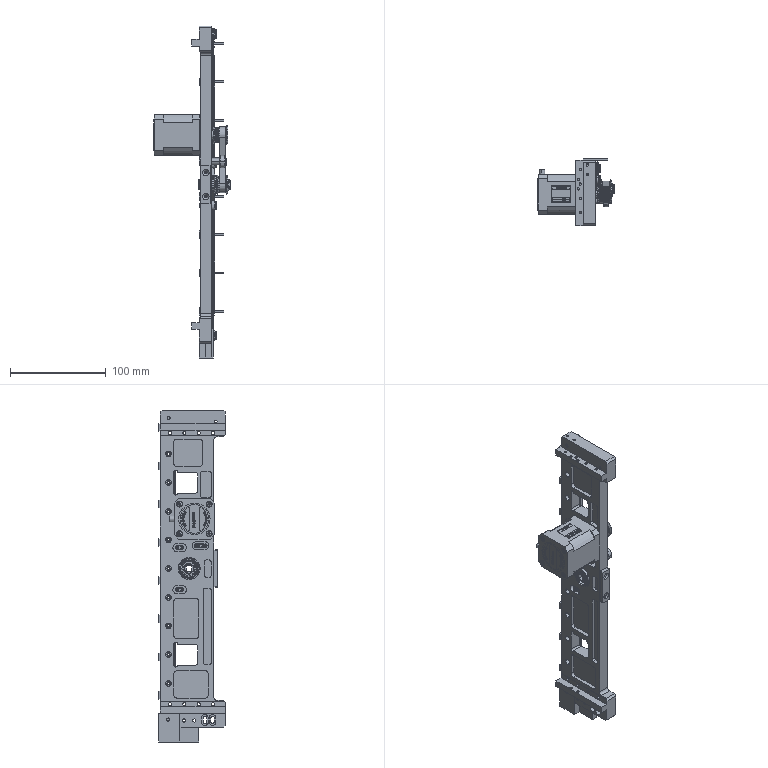Part | NX | features BREP 23 | 45 solids | 4101 faces | volume 279184 mm3 | plane 2068 | cylinder 1273 | spline 403 | cone 153 | sphere 124 | torus 80 | commonest cylinder face diameters 0.46 x382 4 x133 15.66 x80 6 x74 3.4 x68 2.5 x52